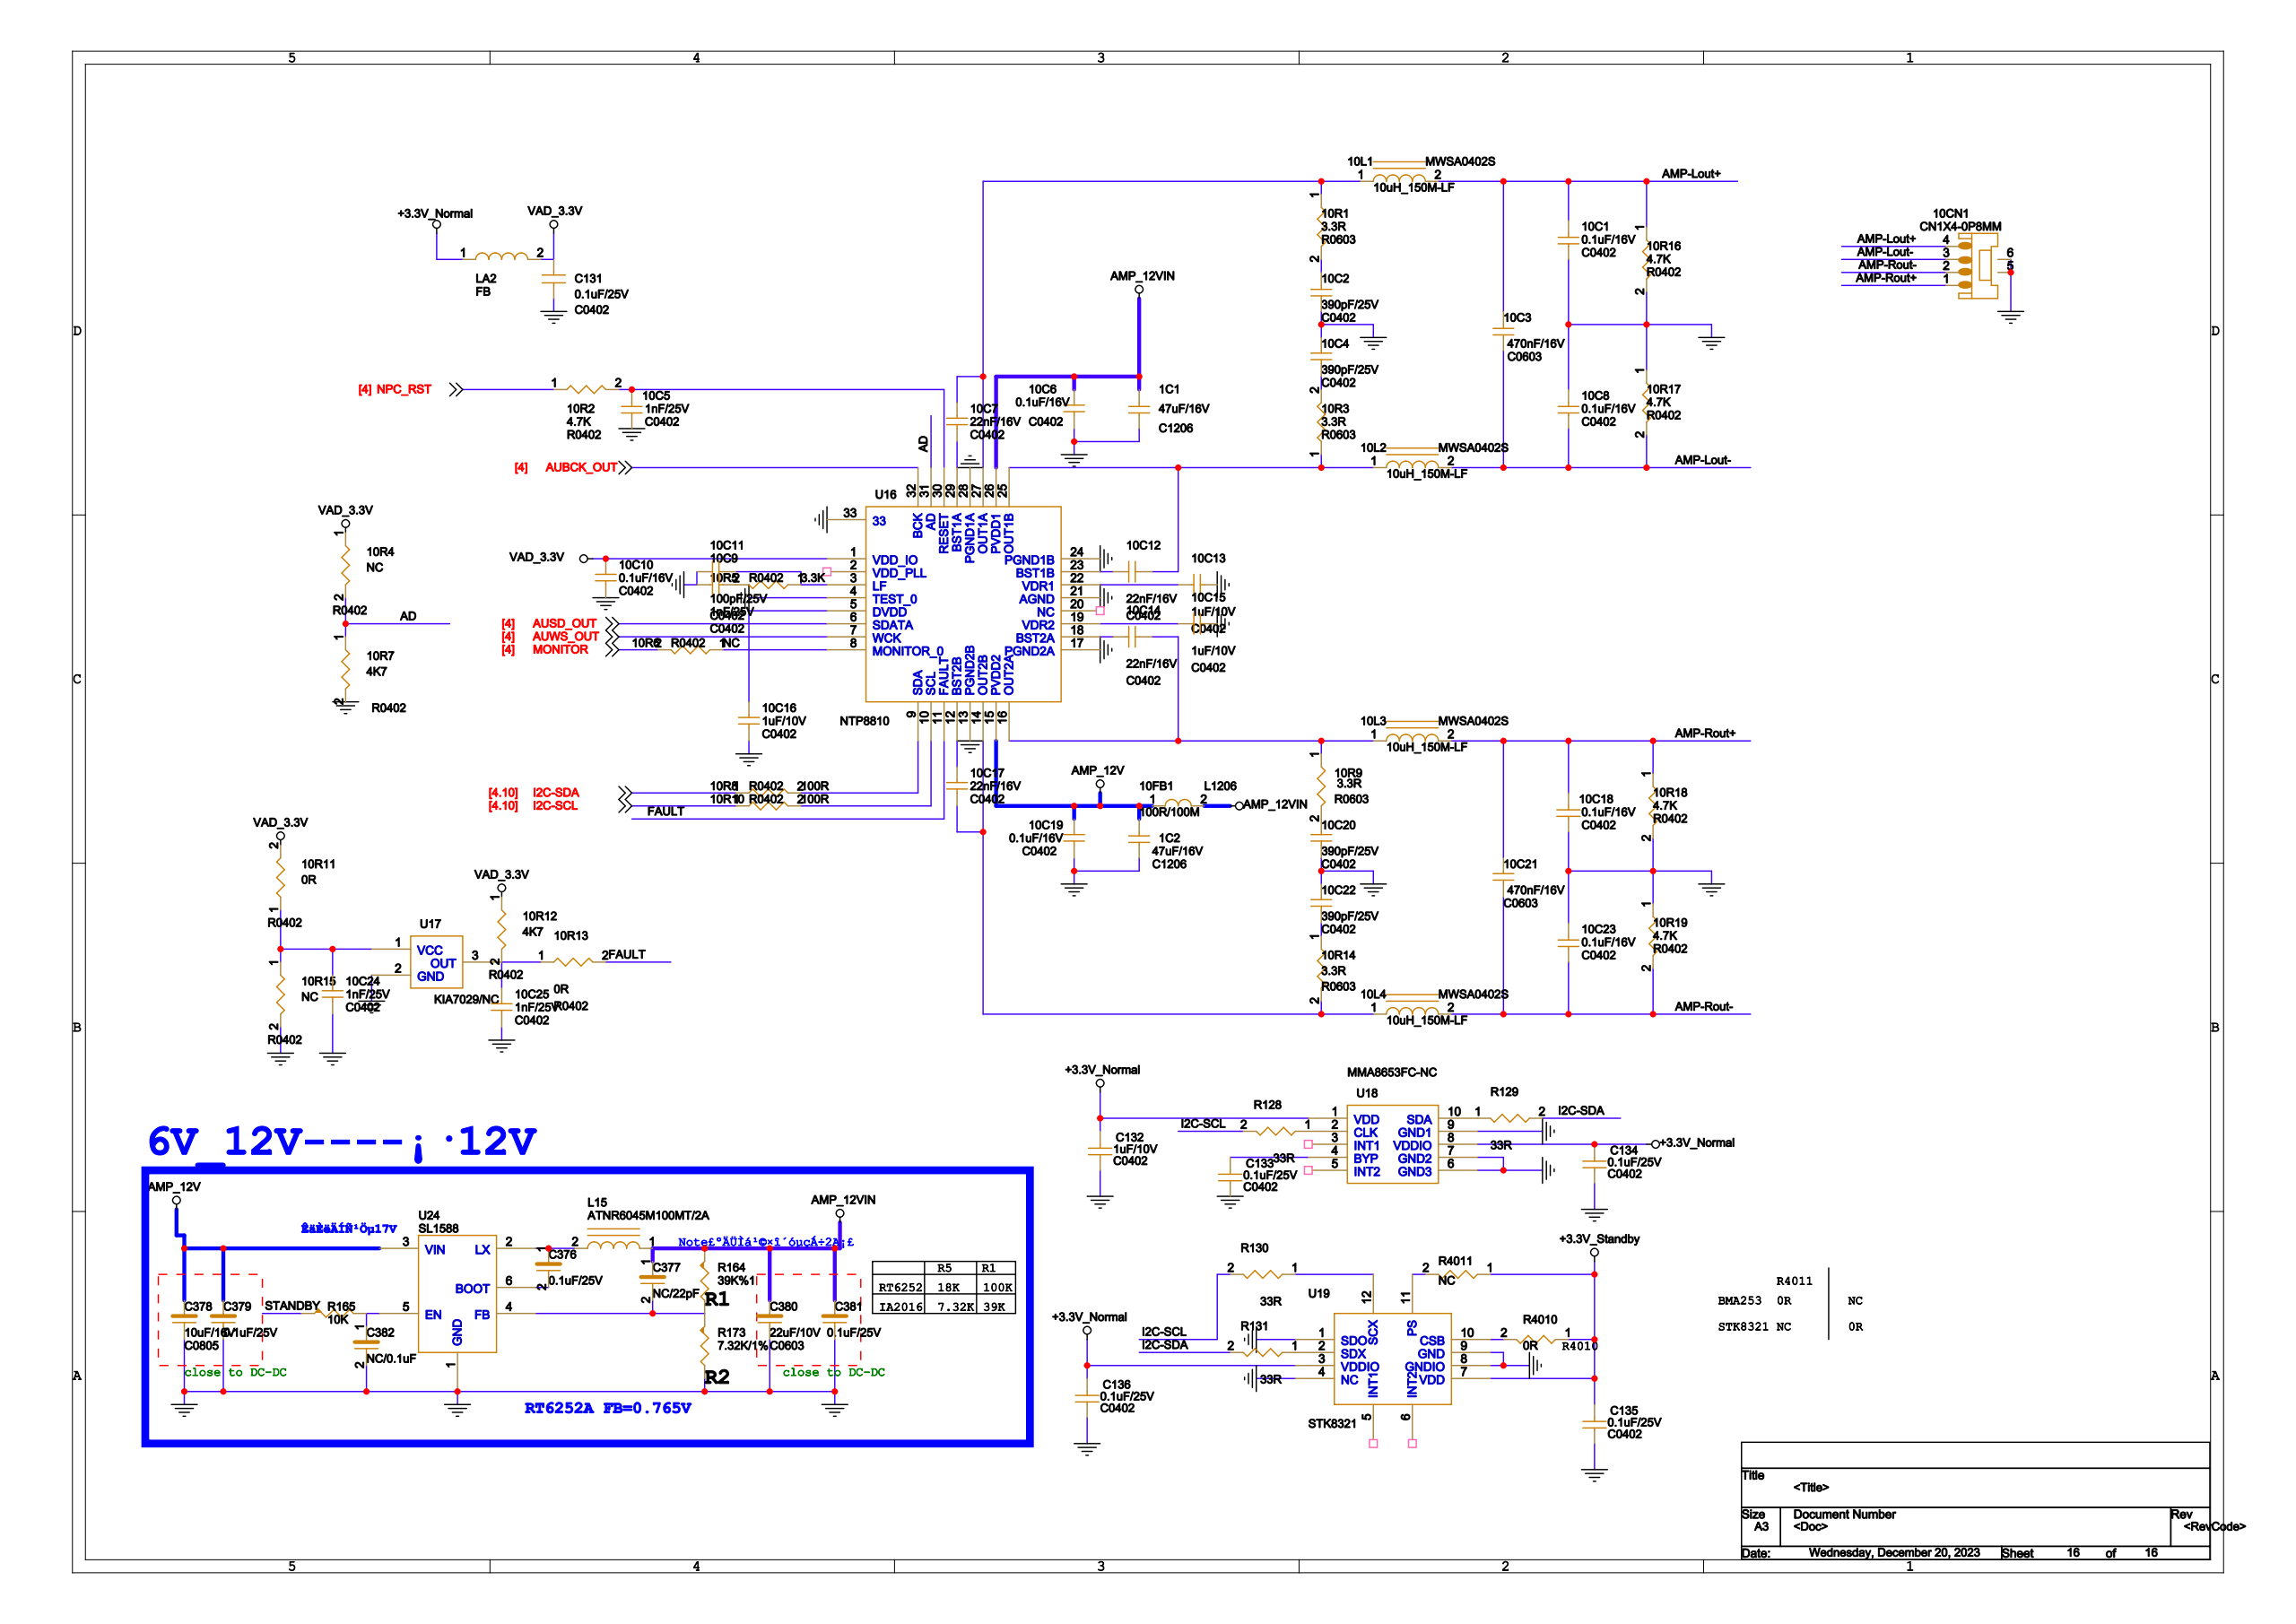Circuit board | Cadence Allegro | 1223 parts | 777 nets | one sheet of the schematic
Parts on this sheet (reference | value | footprint):
1C1 | 47uF/16V | C1206
1C2 | 47uF/16V | C1206
10C1 | 0.1uF/16V | C0402
10C2 | 390pF/25V | C0402
10C3 | 470nF/16V | C0603
10C4 | 390pF/25V | C0402
10C5 | 1nF/25V | C0402
10C6 | 0.1uF/16V | C0402
10C7 | 22nF/16V | C0402
10C8 | 0.1uF/16V | C0402
10C9 | 1nF/25V | C0402
10C10 | 0.1uF/16V | C0402
10C11 | 100pF/25V | C0402
10C12 | 22nF/16V | C0402
10C13 | 1uF/10V | C0402
10C14 | 22nF/16V | C0402
10C15 | 1uF/10V | C0402
10C16 | 1uF/10V | C0402
10C17 | 22nF/16V | C0402
10C18 | 0.1uF/16V | C0402
10C19 | 0.1uF/16V | C0402
10C20 | 390pF/25V | C0402
10C21 | 470nF/16V | C0603
10C22 | 390pF/25V | C0402
10C23 | 0.1uF/16V | C0402
10C24 | 1nF/25V | C0402
10C25 | 1nF/25V | C0402
10CN1 | 4PIN-2.54-L-H-G | CN1X4-0P8MM
10FB1 | 100R/100M | L1206
10L1 | 10uH_150M-LF | MWSA0402S
10L2 | 10uH_150M-LF | MWSA0402S
10L3 | 10uH_150M-LF | MWSA0402S
10L4 | 10uH_150M-LF | MWSA0402S
10R1 | 3.3R | R0603
10R2 | 4.7K | R0402
10R3 | 3.3R | R0603
10R4 | NC | R0402
10R7 | 4K7 | R0402
10R9 | 3.3R | R0603
10R11 | 0R | R0402
10R12 | 4K7 | R0402
10R13 | 0R | R0402
10R14 | 3.3R | R0603
10R15 | NC | R0402
10R16 | 4.7K | R0402
10R17 | 4.7K | R0402
10R18 | 4.7K | R0402
10R19 | 4.7K | R0402
C131 | 0.1uF/25V | C0402
C132 | 1uF/10V | C0402
C133 | 0.1uF/25V | C0402
C134 | 0.1uF/25V | C0402
C135 | 0.1uF/25V | C0402
C136 | 0.1uF/25V | C0402
C376 | 0.1uF/25V | C0402
C377 | NC/22pF | C0402
C378 | 10uF/16V | C0805
C379 | 0.1uF/25V | C0402
C380 | 22uF/10V | C0603
C381 | 0.1uF/25V | C0402
C382 | NC/0.1uF | C0402
L15 | ATNR6045M100MT/2A | MWSA0402S
LA2 | FB | R0805
R128 | 33R | R0402
R129 | 33R | R0402
R130 | 33R | R0402
R131 | 33R | R0402
R164 | 39K%1 | R0402
R165 | 10K | R0402
R173 | 7.32K/1% | R0402
R4010 | 0R | R0402
R4011 | NC | R0402
U16 | NTP8810 | QFN32_5X5MM
U17 | KIA7029/NC | SOT89
U18 | MMA8653FC-NC | DFN10
U19 | STK8321 | LGA12_2X2MM
U24 | SL1588 | SOT-23-6
Nets of these parts (net: part-pin ...):
GND: 1C1-1 1C2-1 10C1-1 10C2-1 10C4-1 10C5-1 10C6-2 10C8-2 10C9-1 10C10-2 10C11-1 10C13-2 10C15-2 10C16-2 10C18-1 10C19-2 10C20-2 10C22-1 10C23-2 10C24-2 10C25-2 10CN1-5 10CN1-6 10R7-2 10R15-2 10R16-2 10R17-1 10R18-2 10R19-1 C131-2 C132-1 C133-1 C134-1 C135-1 C136-1 C378-2 C379-2 C380-2 C381-2 C382-2 R173-2 U17-2 U18-6 U18-7 U18-9 U19-1 U19-4 U19-8 U19-9 U24-1 U16-4 U16-13 U16-17 U16-21 U16-24 U16-28 U16-33
AMP-LOUT+: 10C1-2 10C3-2 10CN1-4 10L1-2 10R16-1
VAD_3.3V: 10C10-1 10R4-1 10R11-2 10R12-1 C131-1 LA2-2 U16-1
AMP_12V: 1C2-2 10C19-1 10FB1-1 C378-1 C379-1 U24-3 U16-15
AMP-ROUT-: 10C21-2 10C23-1 10CN1-2 10L4-2 10R19-2
AMP_12VIN: 1C1-2 10C6-1 10FB1-2 C377-1 C380-1 C381-1 L15-1 R164-1 U16-26
AMP-LOUT-: 10C3-1 10C8-1 10CN1-3 10L2-2 10R17-2
N24194766: 10C11-2 U16-3
N24195194: 10C12-1 U16-23
N24195196: 10C12-2 10L2-1 10R3-1 U16-25
N24195143: 10C14-1 U16-18
N24195145: 10C14-2 10L3-1 10R9-1 U16-16
N24195075: 10C17-1 U16-12
N24195077: 10C17-2 10L4-1 10R14-2 U16-14
N24195250: 10C7-1 10L1-1 10R1-1 U16-27
N24195248: 10C7-2 U16-29
N24195168: 10C13-1 U16-22
N24195166: 10C15-1 U16-19
N24194848: 10C16-1 U16-5
AMP-ROUT+: 10C18-2 10C21-1 10CN1-1 10L3-2 10R18-1
N24195566: 10C2-2 10R1-2
N241953830: 10C20-1 10R9-2
N24195612: 10C22-2 10R14-1
N24195562: 10C4-2 10R3-2
N24195021: 10C24-1 10R11-1 10R15-1 U17-1
N24194969: 10C25-1 10R12-2 10R13-1 U17-3
N24195273: 10C5-2 10R2-2 U16-30
N241947731: 10C9-2
I2C-SCL: R128-2 R130-2
I2C-SDA: R129-2 R131-2
FAULT: 10R13-2 U16-11
AD: 10R4-2 10R7-1 U16-31
NPC_RST: 10R2-1
N25981570: C376-1 L15-2 U24-2
N25981680: C376-2 U24-6
+3.3V_STANDBY: C135-2 R4010-1 R4011-1 U19-7
N25981513: C382-1 R165-2 U24-5
N16947002: C133-2 U18-4
+3.3V_EMMC: C132-2 C134-2 C136-2 LA2-1 U18-1 U18-8 U19-3
N25981651: C377-2 R164-2 R173-1 U24-4
STANDBY: R165-1
N241876281: R128-1 U18-2
N241876289: R129-1 U18-10
N17043535: R130-1 U19-12
N241878190: R131-1 U19-2
N24488866: R4010-2 U19-10
N17052813: R4011-2 U19-11
AUBCK_OUT: U16-32
AUSD_OUT: U16-6
AUWS_OUT: U16-7